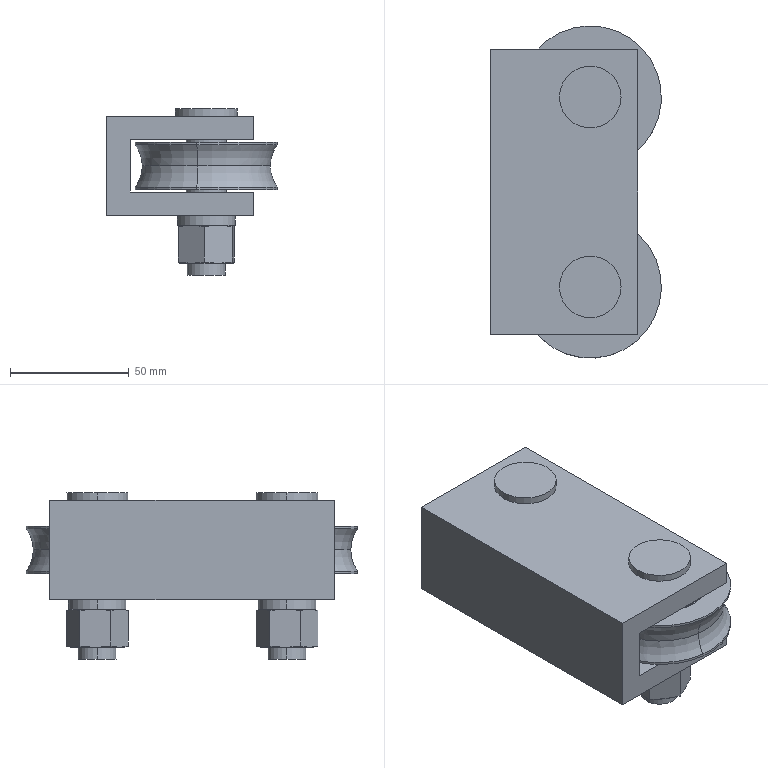Part | SolidWorks | 11 solids | 414 faces | box 72 x 140 x 70 mm | volume 285361 mm3 | cylinder 184 | plane 178 | cone 28 | torus 24 | commonest cylinder face diameters 6.5 x60 22.1 x22 35.1 x22 16 x8 17 x8 17.2 x8